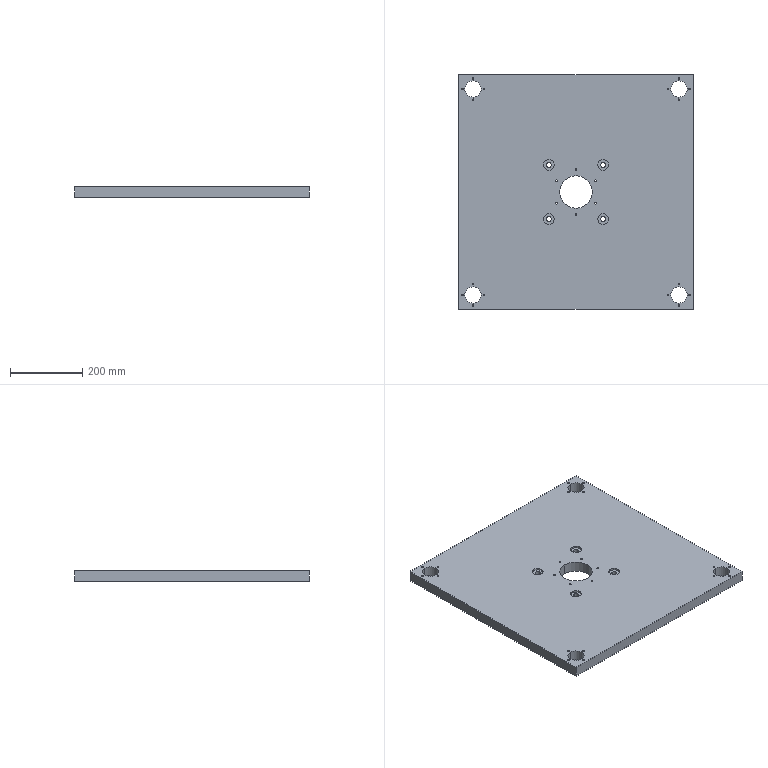Part | SolidWorks | features BaseBody 1 | 1 solid | 92 faces | box 650 x 650 x 30 mm | volume 12242993 mm3 | cylinder 78 | plane 14 | commonest cylinder face diameters 5 x44 13.5 x8 20 x8 30 x8 45 x8 90 x2